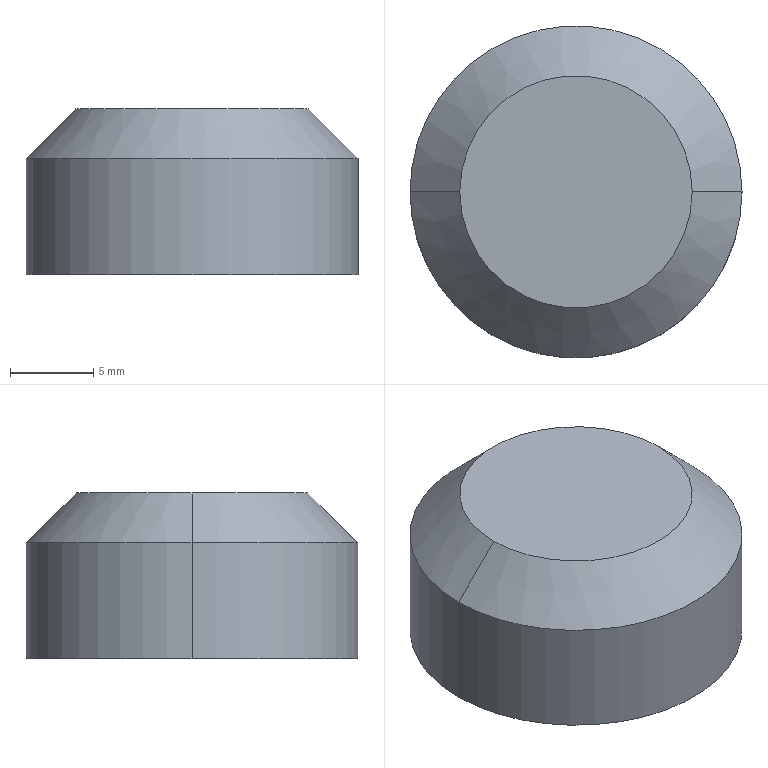Part | STEP file | Cable Carrier Part 4 | 1 solid | 6 faces | box 20 x 20 x 10 mm | volume 2887 mm3 | cone 2 | cylinder 2 | plane 2 | commonest cylinder face diameters 20 x2
STEP:
#1=CARTESIAN_POINT('',(0.,0.,0.));
#2=DIRECTION('',(0.,0.,1.));
#3=DIRECTION('',(1.,0.,0.));
#4=AXIS2_PLACEMENT_3D('',#1,#2,#3);
#5=CARTESIAN_POINT('',(7.,0.,10.));
#6=VERTEX_POINT('',#5);
#7=CARTESIAN_POINT('',(-7.,0.,10.));
#8=VERTEX_POINT('',#7);
#9=CARTESIAN_POINT('',(0.,0.,10.));
#10=DIRECTION('',(0.,0.,1.));
#11=DIRECTION('',(1.,0.,0.));
#12=AXIS2_PLACEMENT_3D('',#9,#10,#11);
#13=CIRCLE('',#12,7.);
#14=CARTESIAN_POINT('',(0.,0.,10.));
#15=DIRECTION('',(0.,0.,-1.));
#16=DIRECTION('',(-1.,0.,0.));
#17=AXIS2_PLACEMENT_3D('',#14,#15,#16);
#18=CONICAL_SURFACE('',#17,7.,0.7854);
#19=CARTESIAN_POINT('',(3.142,0.));
#20=DIRECTION('',(-1.,0.));
#21=VECTOR('',#20,1.);
#22=LINE('',#19,#21);
#23=(GEOMETRIC_REPRESENTATION_CONTEXT(2)PARAMETRIC_REPRESENTATION_CONTEXT()REPRESENTATION_CONTEXT('',''));
#24=DEFINITIONAL_REPRESENTATION('',(#22),#23);
#25=PCURVE('',#18,#24);
#26=CARTESIAN_POINT('',(0.,0.,10.));
#27=DIRECTION('',(0.,0.,1.));
#28=DIRECTION('',(1.,0.,0.));
#29=AXIS2_PLACEMENT_3D('',#26,#27,#28);
#30=PLANE('',#29);
#31=CARTESIAN_POINT('',(0.,0.));
#32=DIRECTION('',(1.,0.));
#33=AXIS2_PLACEMENT_2D('',#31,#32);
#34=CIRCLE('',#33,7.);
#35=(GEOMETRIC_REPRESENTATION_CONTEXT(2)PARAMETRIC_REPRESENTATION_CONTEXT()REPRESENTATION_CONTEXT('',''));
#36=DEFINITIONAL_REPRESENTATION('',(#34),#35);
#37=PCURVE('',#30,#36);
#38=SURFACE_CURVE('',#13,(#25,#37),.PCURVE_S1.);
#39=EDGE_CURVE('',#6,#8,#38,.T.);
#40=ORIENTED_EDGE('',*,*,#39,.F.);
#41=CARTESIAN_POINT('',(10.,0.,7.));
#42=VERTEX_POINT('',#41);
#43=CARTESIAN_POINT('',(7.,0.,10.));
#44=DIRECTION('',(0.7071,0.,-0.7071));
#45=VECTOR('',#44,1.);
#46=LINE('',#43,#45);
#47=CARTESIAN_POINT('',(3.142,0.));
#48=DIRECTION('',(0.,1.));
#49=VECTOR('',#48,1.);
#50=LINE('',#47,#49);
#51=(GEOMETRIC_REPRESENTATION_CONTEXT(2)PARAMETRIC_REPRESENTATION_CONTEXT()REPRESENTATION_CONTEXT('',''));
#52=DEFINITIONAL_REPRESENTATION('',(#50),#51);
#53=PCURVE('',#18,#52);
#54=CARTESIAN_POINT('',(0.,0.,10.));
#55=DIRECTION('',(0.,0.,-1.));
#56=DIRECTION('',(-1.,0.,0.));
#57=AXIS2_PLACEMENT_3D('',#54,#55,#56);
#58=CONICAL_SURFACE('',#57,7.,0.7854);
#59=CARTESIAN_POINT('',(3.142,0.));
#60=DIRECTION('',(0.,1.));
#61=VECTOR('',#60,1.);
#62=LINE('',#59,#61);
#63=(GEOMETRIC_REPRESENTATION_CONTEXT(2)PARAMETRIC_REPRESENTATION_CONTEXT()REPRESENTATION_CONTEXT('',''));
#64=DEFINITIONAL_REPRESENTATION('',(#62),#63);
#65=PCURVE('',#58,#64);
#66=SURFACE_CURVE('',#46,(#53,#65),.PCURVE_S1.);
#67=EDGE_CURVE('',#6,#42,#66,.T.);
#68=ORIENTED_EDGE('',*,*,#67,.T.);
#69=CARTESIAN_POINT('',(-10.,0.,7.));
#70=VERTEX_POINT('',#69);
#71=CARTESIAN_POINT('',(0.,0.,7.));
#72=DIRECTION('',(0.,0.,-1.));
#73=DIRECTION('',(1.,0.,0.));
#74=AXIS2_PLACEMENT_3D('',#71,#72,#73);
#75=CIRCLE('',#74,10.);
#76=CARTESIAN_POINT('',(-3.142,3.));
#77=DIRECTION('',(1.,0.));
#78=VECTOR('',#77,1.);
#79=LINE('',#76,#78);
#80=(GEOMETRIC_REPRESENTATION_CONTEXT(2)PARAMETRIC_REPRESENTATION_CONTEXT()REPRESENTATION_CONTEXT('',''));
#81=DEFINITIONAL_REPRESENTATION('',(#79),#80);
#82=PCURVE('',#18,#81);
#83=CARTESIAN_POINT('',(0.,0.,10.));
#84=DIRECTION('',(0.,0.,-1.));
#85=DIRECTION('',(-1.,0.,0.));
#86=AXIS2_PLACEMENT_3D('',#83,#84,#85);
#87=CYLINDRICAL_SURFACE('',#86,10.);
#88=CARTESIAN_POINT('',(-3.142,3.));
#89=DIRECTION('',(1.,0.));
#90=VECTOR('',#89,1.);
#91=LINE('',#88,#90);
#92=(GEOMETRIC_REPRESENTATION_CONTEXT(2)PARAMETRIC_REPRESENTATION_CONTEXT()REPRESENTATION_CONTEXT('',''));
#93=DEFINITIONAL_REPRESENTATION('',(#91),#92);
#94=PCURVE('',#87,#93);
#95=SURFACE_CURVE('',#75,(#82,#94),.PCURVE_S1.);
#96=EDGE_CURVE('',#70,#42,#95,.T.);
#97=ORIENTED_EDGE('',*,*,#96,.F.);
#98=CARTESIAN_POINT('',(-7.,0.,10.));
#99=DIRECTION('',(-0.7071,0.,-0.7071));
#100=VECTOR('',#99,1.);
#101=LINE('',#98,#100);
#102=CARTESIAN_POINT('',(0.,0.));
#103=DIRECTION('',(0.,1.));
#104=VECTOR('',#103,1.);
#105=LINE('',#102,#104);
#106=(GEOMETRIC_REPRESENTATION_CONTEXT(2)PARAMETRIC_REPRESENTATION_CONTEXT()REPRESENTATION_CONTEXT('',''));
#107=DEFINITIONAL_REPRESENTATION('',(#105),#106);
#108=PCURVE('',#18,#107);
#109=CARTESIAN_POINT('',(6.283,0.));
#110=DIRECTION('',(0.,1.));
#111=VECTOR('',#110,1.);
#112=LINE('',#109,#111);
#113=(GEOMETRIC_REPRESENTATION_CONTEXT(2)PARAMETRIC_REPRESENTATION_CONTEXT()REPRESENTATION_CONTEXT('',''));
#114=DEFINITIONAL_REPRESENTATION('',(#112),#113);
#115=PCURVE('',#58,#114);
#116=SURFACE_CURVE('',#101,(#108,#115),.PCURVE_S1.);
#117=EDGE_CURVE('',#8,#70,#116,.T.);
#118=ORIENTED_EDGE('',*,*,#117,.F.);
#119=EDGE_LOOP('',(#40,#68,#97,#118));
#120=FACE_BOUND('',#119,.T.);
#121=ADVANCED_FACE('',(#120),#18,.T.);
#122=ORIENTED_EDGE('',*,*,#96,.T.);
#123=CARTESIAN_POINT('',(10.,0.,0.));
#124=VERTEX_POINT('',#123);
#125=CARTESIAN_POINT('',(10.,0.,10.));
#126=DIRECTION('',(0.,0.,-1.));
#127=VECTOR('',#126,1.);
#128=LINE('',#125,#127);
#129=CARTESIAN_POINT('',(3.142,0.));
#130=DIRECTION('',(0.,1.));
#131=VECTOR('',#130,1.);
#132=LINE('',#129,#131);
#133=(GEOMETRIC_REPRESENTATION_CONTEXT(2)PARAMETRIC_REPRESENTATION_CONTEXT()REPRESENTATION_CONTEXT('',''));
#134=DEFINITIONAL_REPRESENTATION('',(#132),#133);
#135=PCURVE('',#87,#134);
#136=CARTESIAN_POINT('',(0.,0.,10.));
#137=DIRECTION('',(0.,0.,-1.));
#138=DIRECTION('',(-1.,0.,0.));
#139=AXIS2_PLACEMENT_3D('',#136,#137,#138);
#140=CYLINDRICAL_SURFACE('',#139,10.);
#141=CARTESIAN_POINT('',(3.142,0.));
#142=DIRECTION('',(0.,1.));
#143=VECTOR('',#142,1.);
#144=LINE('',#141,#143);
#145=(GEOMETRIC_REPRESENTATION_CONTEXT(2)PARAMETRIC_REPRESENTATION_CONTEXT()REPRESENTATION_CONTEXT('',''));
#146=DEFINITIONAL_REPRESENTATION('',(#144),#145);
#147=PCURVE('',#140,#146);
#148=SURFACE_CURVE('',#128,(#135,#147),.PCURVE_S1.);
#149=EDGE_CURVE('',#42,#124,#148,.T.);
#150=ORIENTED_EDGE('',*,*,#149,.T.);
#151=CARTESIAN_POINT('',(-10.,0.,0.));
#152=VERTEX_POINT('',#151);
#153=CARTESIAN_POINT('',(0.,0.,0.));
#154=DIRECTION('',(0.,0.,1.));
#155=DIRECTION('',(1.,0.,0.));
#156=AXIS2_PLACEMENT_3D('',#153,#154,#155);
#157=CIRCLE('',#156,10.);
#158=CARTESIAN_POINT('',(3.142,10.));
#159=DIRECTION('',(-1.,0.));
#160=VECTOR('',#159,1.);
#161=LINE('',#158,#160);
#162=(GEOMETRIC_REPRESENTATION_CONTEXT(2)PARAMETRIC_REPRESENTATION_CONTEXT()REPRESENTATION_CONTEXT('',''));
#163=DEFINITIONAL_REPRESENTATION('',(#161),#162);
#164=PCURVE('',#87,#163);
#165=CARTESIAN_POINT('',(0.,0.,0.));
#166=DIRECTION('',(0.,0.,1.));
#167=DIRECTION('',(1.,0.,0.));
#168=AXIS2_PLACEMENT_3D('',#165,#166,#167);
#169=PLANE('',#168);
#170=CARTESIAN_POINT('',(0.,0.));
#171=DIRECTION('',(1.,0.));
#172=AXIS2_PLACEMENT_2D('',#170,#171);
#173=CIRCLE('',#172,10.);
#174=(GEOMETRIC_REPRESENTATION_CONTEXT(2)PARAMETRIC_REPRESENTATION_CONTEXT()REPRESENTATION_CONTEXT('',''));
#175=DEFINITIONAL_REPRESENTATION('',(#173),#174);
#176=PCURVE('',#169,#175);
#177=SURFACE_CURVE('',#157,(#164,#176),.PCURVE_S1.);
#178=EDGE_CURVE('',#124,#152,#177,.T.);
#179=ORIENTED_EDGE('',*,*,#178,.T.);
#180=CARTESIAN_POINT('',(-10.,0.,10.));
#181=DIRECTION('',(0.,0.,-1.));
#182=VECTOR('',#181,1.);
#183=LINE('',#180,#182);
#184=CARTESIAN_POINT('',(0.,0.));
#185=DIRECTION('',(0.,1.));
#186=VECTOR('',#185,1.);
#187=LINE('',#184,#186);
#188=(GEOMETRIC_REPRESENTATION_CONTEXT(2)PARAMETRIC_REPRESENTATION_CONTEXT()REPRESENTATION_CONTEXT('',''));
#189=DEFINITIONAL_REPRESENTATION('',(#187),#188);
#190=PCURVE('',#87,#189);
#191=CARTESIAN_POINT('',(6.283,0.));
#192=DIRECTION('',(0.,1.));
#193=VECTOR('',#192,1.);
#194=LINE('',#191,#193);
#195=(GEOMETRIC_REPRESENTATION_CONTEXT(2)PARAMETRIC_REPRESENTATION_CONTEXT()REPRESENTATION_CONTEXT('',''));
#196=DEFINITIONAL_REPRESENTATION('',(#194),#195);
#197=PCURVE('',#140,#196);
#198=SURFACE_CURVE('',#183,(#190,#197),.PCURVE_S1.);
#199=EDGE_CURVE('',#70,#152,#198,.T.);
#200=ORIENTED_EDGE('',*,*,#199,.F.);
#201=EDGE_LOOP('',(#122,#150,#179,#200));
#202=FACE_BOUND('',#201,.T.);
#203=ADVANCED_FACE('',(#202),#87,.T.);
#204=ORIENTED_EDGE('',*,*,#149,.F.);
#205=CARTESIAN_POINT('',(0.,0.,7.));
#206=DIRECTION('',(0.,0.,-1.));
#207=DIRECTION('',(1.,0.,0.));
#208=AXIS2_PLACEMENT_3D('',#205,#206,#207);
#209=CIRCLE('',#208,10.);
#210=CARTESIAN_POINT('',(3.142,3.));
#211=DIRECTION('',(1.,0.));
#212=VECTOR('',#211,1.);
#213=LINE('',#210,#212);
#214=(GEOMETRIC_REPRESENTATION_CONTEXT(2)PARAMETRIC_REPRESENTATION_CONTEXT()REPRESENTATION_CONTEXT('',''));
#215=DEFINITIONAL_REPRESENTATION('',(#213),#214);
#216=PCURVE('',#140,#215);
#217=CARTESIAN_POINT('',(3.142,3.));
#218=DIRECTION('',(1.,0.));
#219=VECTOR('',#218,1.);
#220=LINE('',#217,#219);
#221=(GEOMETRIC_REPRESENTATION_CONTEXT(2)PARAMETRIC_REPRESENTATION_CONTEXT()REPRESENTATION_CONTEXT('',''));
#222=DEFINITIONAL_REPRESENTATION('',(#220),#221);
#223=PCURVE('',#58,#222);
#224=SURFACE_CURVE('',#209,(#216,#223),.PCURVE_S1.);
#225=EDGE_CURVE('',#42,#70,#224,.T.);
#226=ORIENTED_EDGE('',*,*,#225,.T.);
#227=ORIENTED_EDGE('',*,*,#199,.T.);
#228=CARTESIAN_POINT('',(0.,0.,0.));
#229=DIRECTION('',(0.,0.,1.));
#230=DIRECTION('',(1.,0.,0.));
#231=AXIS2_PLACEMENT_3D('',#228,#229,#230);
#232=CIRCLE('',#231,10.);
#233=CARTESIAN_POINT('',(9.425,10.));
#234=DIRECTION('',(-1.,0.));
#235=VECTOR('',#234,1.);
#236=LINE('',#233,#235);
#237=(GEOMETRIC_REPRESENTATION_CONTEXT(2)PARAMETRIC_REPRESENTATION_CONTEXT()REPRESENTATION_CONTEXT('',''));
#238=DEFINITIONAL_REPRESENTATION('',(#236),#237);
#239=PCURVE('',#140,#238);
#240=CARTESIAN_POINT('',(0.,0.));
#241=DIRECTION('',(1.,0.));
#242=AXIS2_PLACEMENT_2D('',#240,#241);
#243=CIRCLE('',#242,10.);
#244=(GEOMETRIC_REPRESENTATION_CONTEXT(2)PARAMETRIC_REPRESENTATION_CONTEXT()REPRESENTATION_CONTEXT('',''));
#245=DEFINITIONAL_REPRESENTATION('',(#243),#244);
#246=PCURVE('',#169,#245);
#247=SURFACE_CURVE('',#232,(#239,#246),.PCURVE_S1.);
#248=EDGE_CURVE('',#152,#124,#247,.T.);
#249=ORIENTED_EDGE('',*,*,#248,.T.);
#250=EDGE_LOOP('',(#204,#226,#227,#249));
#251=FACE_BOUND('',#250,.T.);
#252=ADVANCED_FACE('',(#251),#140,.T.);
#253=CARTESIAN_POINT('',(0.,0.,10.));
#254=DIRECTION('',(0.,0.,1.));
#255=DIRECTION('',(1.,0.,0.));
#256=AXIS2_PLACEMENT_3D('',#253,#254,#255);
#257=CIRCLE('',#256,7.);
#258=CARTESIAN_POINT('',(0.,0.));
#259=DIRECTION('',(1.,0.));
#260=AXIS2_PLACEMENT_2D('',#258,#259);
#261=CIRCLE('',#260,7.);
#262=(GEOMETRIC_REPRESENTATION_CONTEXT(2)PARAMETRIC_REPRESENTATION_CONTEXT()REPRESENTATION_CONTEXT('',''));
#263=DEFINITIONAL_REPRESENTATION('',(#261),#262);
#264=PCURVE('',#30,#263);
#265=CARTESIAN_POINT('',(9.425,0.));
#266=DIRECTION('',(-1.,0.));
#267=VECTOR('',#266,1.);
#268=LINE('',#265,#267);
#269=(GEOMETRIC_REPRESENTATION_CONTEXT(2)PARAMETRIC_REPRESENTATION_CONTEXT()REPRESENTATION_CONTEXT('',''));
#270=DEFINITIONAL_REPRESENTATION('',(#268),#269);
#271=PCURVE('',#58,#270);
#272=SURFACE_CURVE('',#257,(#264,#271),.PCURVE_S1.);
#273=EDGE_CURVE('',#8,#6,#272,.T.);
#274=ORIENTED_EDGE('',*,*,#273,.T.);
#275=ORIENTED_EDGE('',*,*,#39,.T.);
#276=EDGE_LOOP('',(#274,#275));
#277=FACE_BOUND('',#276,.T.);
#278=ADVANCED_FACE('',(#277),#30,.T.);
#279=ORIENTED_EDGE('',*,*,#248,.F.);
#280=ORIENTED_EDGE('',*,*,#178,.F.);
#281=EDGE_LOOP('',(#279,#280));
#282=FACE_BOUND('',#281,.T.);
#283=ADVANCED_FACE('',(#282),#169,.F.);
#284=ORIENTED_EDGE('',*,*,#67,.F.);
#285=ORIENTED_EDGE('',*,*,#273,.F.);
#286=ORIENTED_EDGE('',*,*,#117,.T.);
#287=ORIENTED_EDGE('',*,*,#225,.F.);
#288=EDGE_LOOP('',(#284,#285,#286,#287));
#289=FACE_BOUND('',#288,.T.);
#290=ADVANCED_FACE('',(#289),#58,.T.);
#291=CLOSED_SHELL('',(#121,#203,#252,#278,#283,#290));
#292=MANIFOLD_SOLID_BREP('',#291);
#293=(LENGTH_UNIT()NAMED_UNIT(*)SI_UNIT(.MILLI.,.METRE.));
#294=UNCERTAINTY_MEASURE_WITH_UNIT(LENGTH_MEASURE(0.0000001),#293,'','');
#295=(NAMED_UNIT(*)PLANE_ANGLE_UNIT()SI_UNIT($,.RADIAN.));
#296=(NAMED_UNIT(*)SI_UNIT($,.STERADIAN.)SOLID_ANGLE_UNIT());
#297=(GEOMETRIC_REPRESENTATION_CONTEXT(3)GLOBAL_UNCERTAINTY_ASSIGNED_CONTEXT((#294))GLOBAL_UNIT_ASSIGNED_CONTEXT((#293,#295,#296))REPRESENTATION_CONTEXT('',''));
#298=ADVANCED_BREP_SHAPE_REPRESENTATION('',(#4,#292),#297);